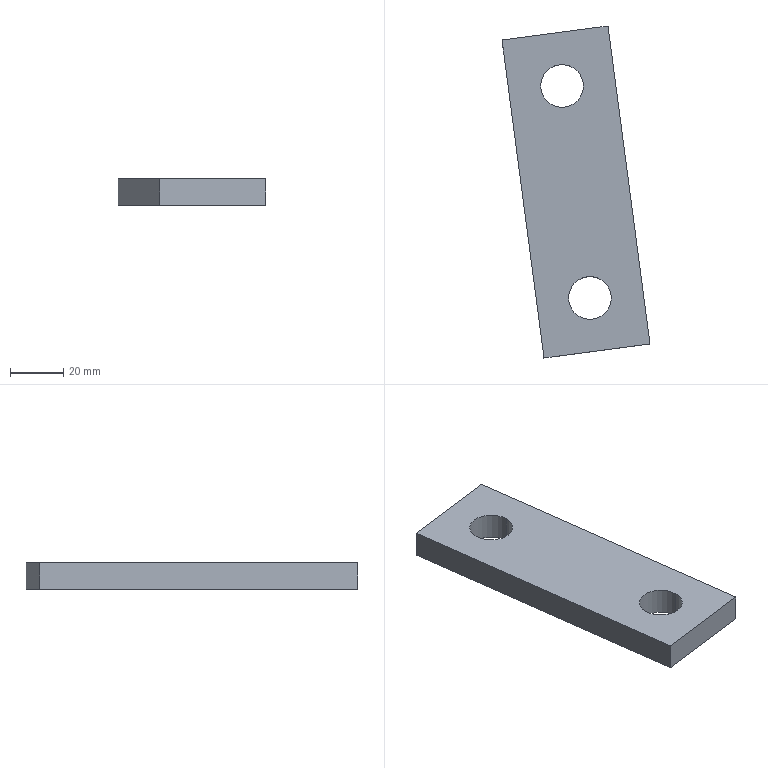Part | SolidWorks | features Extrusion 1 | 1 solid | 10 faces | box 55.334 x 124.197 x 10 mm | volume 43979 mm3 | plane 6 | cylinder 4 | commonest cylinder face diameters 16 x4
STEP:
#1=CARTESIAN_POINT('',(5154.359,2207.673,10.));
#2=VERTEX_POINT('',#1);
#3=CARTESIAN_POINT('',(5170.359,2207.673,10.));
#4=VERTEX_POINT('',#3);
#5=CARTESIAN_POINT('',(5162.359,2207.673,10.));
#6=DIRECTION('',(0.,0.,1.));
#7=DIRECTION('',(-1.,0.,0.));
#8=AXIS2_PLACEMENT_3D('',#5,#6,#7);
#9=CIRCLE('',#8,8.);
#10=EDGE_CURVE('',#2,#4,#9,.T.);
#11=ORIENTED_EDGE('',*,*,#10,.T.);
#12=CARTESIAN_POINT('',(5170.359,2207.673,0.));
#13=VERTEX_POINT('',#12);
#14=CARTESIAN_POINT('',(5170.359,2207.673,10.));
#15=DIRECTION('',(0.,0.,-1.));
#16=VECTOR('',#15,1000.);
#17=LINE('',#14,#16);
#18=EDGE_CURVE('',#4,#13,#17,.T.);
#19=ORIENTED_EDGE('',*,*,#18,.T.);
#20=CARTESIAN_POINT('',(5154.359,2207.673,0.));
#21=VERTEX_POINT('',#20);
#22=CARTESIAN_POINT('',(5162.359,2207.673,0.));
#23=DIRECTION('',(0.,0.,1.));
#24=DIRECTION('',(-1.,0.,0.));
#25=AXIS2_PLACEMENT_3D('',#22,#23,#24);
#26=CIRCLE('',#25,8.);
#27=EDGE_CURVE('',#21,#13,#26,.T.);
#28=ORIENTED_EDGE('',*,*,#27,.F.);
#29=CARTESIAN_POINT('',(5154.359,2207.673,10.));
#30=DIRECTION('',(0.,0.,-1.));
#31=VECTOR('',#30,1000.);
#32=LINE('',#29,#31);
#33=EDGE_CURVE('',#2,#21,#32,.T.);
#34=ORIENTED_EDGE('',*,*,#33,.F.);
#35=EDGE_LOOP('',(#11,#19,#28,#34));
#36=FACE_OUTER_BOUND('',#35,.T.);
#37=CARTESIAN_POINT('',(5162.359,2207.673,10.));
#38=DIRECTION('',(0.,0.,-1.));
#39=DIRECTION('',(-1.,0.,0.));
#40=AXIS2_PLACEMENT_3D('',#37,#38,#39);
#41=CYLINDRICAL_SURFACE('',#40,8.);
#42=ADVANCED_FACE('',(#36),#41,.F.);
#43=CARTESIAN_POINT('',(5143.908,2286.987,10.));
#44=VERTEX_POINT('',#43);
#45=CARTESIAN_POINT('',(5159.908,2286.987,10.));
#46=VERTEX_POINT('',#45);
#47=CARTESIAN_POINT('',(5151.908,2286.987,10.));
#48=DIRECTION('',(0.,0.,1.));
#49=DIRECTION('',(1.,0.,0.));
#50=AXIS2_PLACEMENT_3D('',#47,#48,#49);
#51=CIRCLE('',#50,8.);
#52=EDGE_CURVE('',#44,#46,#51,.T.);
#53=ORIENTED_EDGE('',*,*,#52,.T.);
#54=CARTESIAN_POINT('',(5159.908,2286.987,0.));
#55=VERTEX_POINT('',#54);
#56=CARTESIAN_POINT('',(5159.908,2286.987,10.));
#57=DIRECTION('',(0.,0.,-1.));
#58=VECTOR('',#57,1000.);
#59=LINE('',#56,#58);
#60=EDGE_CURVE('',#46,#55,#59,.T.);
#61=ORIENTED_EDGE('',*,*,#60,.T.);
#62=CARTESIAN_POINT('',(5143.908,2286.987,0.));
#63=VERTEX_POINT('',#62);
#64=CARTESIAN_POINT('',(5151.908,2286.987,0.));
#65=DIRECTION('',(0.,0.,1.));
#66=DIRECTION('',(1.,0.,0.));
#67=AXIS2_PLACEMENT_3D('',#64,#65,#66);
#68=CIRCLE('',#67,8.);
#69=EDGE_CURVE('',#63,#55,#68,.T.);
#70=ORIENTED_EDGE('',*,*,#69,.F.);
#71=CARTESIAN_POINT('',(5143.908,2286.987,10.));
#72=DIRECTION('',(0.,0.,-1.));
#73=VECTOR('',#72,1000.);
#74=LINE('',#71,#73);
#75=EDGE_CURVE('',#44,#63,#74,.T.);
#76=ORIENTED_EDGE('',*,*,#75,.F.);
#77=EDGE_LOOP('',(#53,#61,#70,#76));
#78=FACE_OUTER_BOUND('',#77,.T.);
#79=CARTESIAN_POINT('',(5151.908,2286.987,10.));
#80=DIRECTION('',(0.,0.,-1.));
#81=DIRECTION('',(-1.,0.,0.));
#82=AXIS2_PLACEMENT_3D('',#79,#80,#81);
#83=CYLINDRICAL_SURFACE('',#82,8.);
#84=ADVANCED_FACE('',(#78),#83,.F.);
#85=CARTESIAN_POINT('',(5129.467,2304.203,10.));
#86=VERTEX_POINT('',#85);
#87=CARTESIAN_POINT('',(5145.143,2185.231,10.));
#88=VERTEX_POINT('',#87);
#89=CARTESIAN_POINT('',(5145.143,2185.231,10.));
#90=DIRECTION('',(0.1306,-0.9914,0.));
#91=VECTOR('',#90,1000.);
#92=LINE('',#89,#91);
#93=EDGE_CURVE('',#86,#88,#92,.T.);
#94=ORIENTED_EDGE('',*,*,#93,.T.);
#95=CARTESIAN_POINT('',(5184.801,2190.457,10.));
#96=VERTEX_POINT('',#95);
#97=CARTESIAN_POINT('',(5184.801,2190.457,10.));
#98=DIRECTION('',(0.9914,0.1306,0.));
#99=VECTOR('',#98,1000.);
#100=LINE('',#97,#99);
#101=EDGE_CURVE('',#88,#96,#100,.T.);
#102=ORIENTED_EDGE('',*,*,#101,.T.);
#103=CARTESIAN_POINT('',(5169.124,2309.428,10.));
#104=VERTEX_POINT('',#103);
#105=CARTESIAN_POINT('',(5169.124,2309.428,10.));
#106=DIRECTION('',(-0.1306,0.9914,0.));
#107=VECTOR('',#106,1000.);
#108=LINE('',#105,#107);
#109=EDGE_CURVE('',#96,#104,#108,.T.);
#110=ORIENTED_EDGE('',*,*,#109,.T.);
#111=CARTESIAN_POINT('',(5129.467,2304.203,10.));
#112=DIRECTION('',(-0.9914,-0.1306,0.));
#113=VECTOR('',#112,1000.);
#114=LINE('',#111,#113);
#115=EDGE_CURVE('',#104,#86,#114,.T.);
#116=ORIENTED_EDGE('',*,*,#115,.T.);
#117=EDGE_LOOP('',(#94,#102,#110,#116));
#118=FACE_OUTER_BOUND('',#117,.T.);
#119=ORIENTED_EDGE('',*,*,#52,.F.);
#120=CARTESIAN_POINT('',(5151.908,2286.987,10.));
#121=DIRECTION('',(0.,0.,1.));
#122=DIRECTION('',(1.,0.,0.));
#123=AXIS2_PLACEMENT_3D('',#120,#121,#122);
#124=CIRCLE('',#123,8.);
#125=EDGE_CURVE('',#46,#44,#124,.T.);
#126=ORIENTED_EDGE('',*,*,#125,.F.);
#127=EDGE_LOOP('',(#119,#126));
#128=FACE_BOUND('',#127,.T.);
#129=ORIENTED_EDGE('',*,*,#10,.F.);
#130=CARTESIAN_POINT('',(5162.359,2207.673,10.));
#131=DIRECTION('',(0.,0.,1.));
#132=DIRECTION('',(-1.,0.,0.));
#133=AXIS2_PLACEMENT_3D('',#130,#131,#132);
#134=CIRCLE('',#133,8.);
#135=EDGE_CURVE('',#4,#2,#134,.T.);
#136=ORIENTED_EDGE('',*,*,#135,.F.);
#137=EDGE_LOOP('',(#129,#136));
#138=FACE_BOUND('',#137,.T.);
#139=CARTESIAN_POINT('',(0.,0.,10.));
#140=DIRECTION('',(0.,0.,-1.));
#141=DIRECTION('',(-1.,0.,0.));
#142=AXIS2_PLACEMENT_3D('',#139,#140,#141);
#143=PLANE('',#142);
#144=ADVANCED_FACE('',(#118,#128,#138),#143,.F.);
#145=ORIENTED_EDGE('',*,*,#69,.T.);
#146=CARTESIAN_POINT('',(5151.908,2286.987,0.));
#147=DIRECTION('',(0.,0.,1.));
#148=DIRECTION('',(1.,0.,0.));
#149=AXIS2_PLACEMENT_3D('',#146,#147,#148);
#150=CIRCLE('',#149,8.);
#151=EDGE_CURVE('',#55,#63,#150,.T.);
#152=ORIENTED_EDGE('',*,*,#151,.T.);
#153=EDGE_LOOP('',(#145,#152));
#154=FACE_BOUND('',#153,.T.);
#155=CARTESIAN_POINT('',(5145.143,2185.231,0.));
#156=VERTEX_POINT('',#155);
#157=CARTESIAN_POINT('',(5184.801,2190.457,0.));
#158=VERTEX_POINT('',#157);
#159=CARTESIAN_POINT('',(5184.801,2190.457,0.));
#160=DIRECTION('',(0.9914,0.1306,0.));
#161=VECTOR('',#160,1000.);
#162=LINE('',#159,#161);
#163=EDGE_CURVE('',#156,#158,#162,.T.);
#164=ORIENTED_EDGE('',*,*,#163,.F.);
#165=CARTESIAN_POINT('',(5129.467,2304.203,0.));
#166=VERTEX_POINT('',#165);
#167=CARTESIAN_POINT('',(5137.305,2244.717,0.));
#168=DIRECTION('',(0.1306,-0.9914,0.));
#169=VECTOR('',#168,1000.);
#170=LINE('',#167,#169);
#171=EDGE_CURVE('',#166,#156,#170,.T.);
#172=ORIENTED_EDGE('',*,*,#171,.F.);
#173=CARTESIAN_POINT('',(5169.124,2309.428,0.));
#174=VERTEX_POINT('',#173);
#175=CARTESIAN_POINT('',(5129.467,2304.203,0.));
#176=DIRECTION('',(-0.9914,-0.1306,0.));
#177=VECTOR('',#176,1000.);
#178=LINE('',#175,#177);
#179=EDGE_CURVE('',#174,#166,#178,.T.);
#180=ORIENTED_EDGE('',*,*,#179,.F.);
#181=CARTESIAN_POINT('',(5169.124,2309.428,0.));
#182=DIRECTION('',(-0.1306,0.9914,0.));
#183=VECTOR('',#182,1000.);
#184=LINE('',#181,#183);
#185=EDGE_CURVE('',#158,#174,#184,.T.);
#186=ORIENTED_EDGE('',*,*,#185,.F.);
#187=EDGE_LOOP('',(#164,#172,#180,#186));
#188=FACE_OUTER_BOUND('',#187,.T.);
#189=ORIENTED_EDGE('',*,*,#27,.T.);
#190=CARTESIAN_POINT('',(5162.359,2207.673,0.));
#191=DIRECTION('',(0.,0.,1.));
#192=DIRECTION('',(-1.,0.,0.));
#193=AXIS2_PLACEMENT_3D('',#190,#191,#192);
#194=CIRCLE('',#193,8.);
#195=EDGE_CURVE('',#13,#21,#194,.T.);
#196=ORIENTED_EDGE('',*,*,#195,.T.);
#197=EDGE_LOOP('',(#189,#196));
#198=FACE_BOUND('',#197,.T.);
#199=CARTESIAN_POINT('',(0.,0.,0.));
#200=DIRECTION('',(0.,0.,-1.));
#201=DIRECTION('',(-1.,0.,0.));
#202=AXIS2_PLACEMENT_3D('',#199,#200,#201);
#203=PLANE('',#202);
#204=ADVANCED_FACE('',(#154,#188,#198),#203,.T.);
#205=ORIENTED_EDGE('',*,*,#163,.T.);
#206=CARTESIAN_POINT('',(5184.801,2190.457,10.));
#207=DIRECTION('',(0.,0.,-1.));
#208=VECTOR('',#207,1000.);
#209=LINE('',#206,#208);
#210=EDGE_CURVE('',#96,#158,#209,.T.);
#211=ORIENTED_EDGE('',*,*,#210,.F.);
#212=ORIENTED_EDGE('',*,*,#101,.F.);
#213=CARTESIAN_POINT('',(5145.143,2185.231,10.));
#214=DIRECTION('',(0.,0.,-1.));
#215=VECTOR('',#214,1000.);
#216=LINE('',#213,#215);
#217=EDGE_CURVE('',#88,#156,#216,.T.);
#218=ORIENTED_EDGE('',*,*,#217,.T.);
#219=EDGE_LOOP('',(#205,#211,#212,#218));
#220=FACE_OUTER_BOUND('',#219,.T.);
#221=CARTESIAN_POINT('',(5184.801,2190.457,10.));
#222=DIRECTION('',(-0.1306,0.9914,0.));
#223=DIRECTION('',(-0.9914,-0.1306,0.));
#224=AXIS2_PLACEMENT_3D('',#221,#222,#223);
#225=PLANE('',#224);
#226=ADVANCED_FACE('',(#220),#225,.F.);
#227=ORIENTED_EDGE('',*,*,#185,.T.);
#228=CARTESIAN_POINT('',(5169.124,2309.428,10.));
#229=DIRECTION('',(0.,0.,-1.));
#230=VECTOR('',#229,1000.);
#231=LINE('',#228,#230);
#232=EDGE_CURVE('',#104,#174,#231,.T.);
#233=ORIENTED_EDGE('',*,*,#232,.F.);
#234=ORIENTED_EDGE('',*,*,#109,.F.);
#235=ORIENTED_EDGE('',*,*,#210,.T.);
#236=EDGE_LOOP('',(#227,#233,#234,#235));
#237=FACE_OUTER_BOUND('',#236,.T.);
#238=CARTESIAN_POINT('',(5169.124,2309.428,10.));
#239=DIRECTION('',(-0.9914,-0.1306,0.));
#240=DIRECTION('',(0.1306,-0.9914,0.));
#241=AXIS2_PLACEMENT_3D('',#238,#239,#240);
#242=PLANE('',#241);
#243=ADVANCED_FACE('',(#237),#242,.F.);
#244=ORIENTED_EDGE('',*,*,#179,.T.);
#245=CARTESIAN_POINT('',(5129.467,2304.203,10.));
#246=DIRECTION('',(0.,0.,-1.));
#247=VECTOR('',#246,1000.);
#248=LINE('',#245,#247);
#249=EDGE_CURVE('',#86,#166,#248,.T.);
#250=ORIENTED_EDGE('',*,*,#249,.F.);
#251=ORIENTED_EDGE('',*,*,#115,.F.);
#252=ORIENTED_EDGE('',*,*,#232,.T.);
#253=EDGE_LOOP('',(#244,#250,#251,#252));
#254=FACE_OUTER_BOUND('',#253,.T.);
#255=CARTESIAN_POINT('',(5129.467,2304.203,10.));
#256=DIRECTION('',(0.1306,-0.9914,0.));
#257=DIRECTION('',(0.9914,0.1306,0.));
#258=AXIS2_PLACEMENT_3D('',#255,#256,#257);
#259=PLANE('',#258);
#260=ADVANCED_FACE('',(#254),#259,.F.);
#261=ORIENTED_EDGE('',*,*,#171,.T.);
#262=ORIENTED_EDGE('',*,*,#217,.F.);
#263=ORIENTED_EDGE('',*,*,#93,.F.);
#264=ORIENTED_EDGE('',*,*,#249,.T.);
#265=EDGE_LOOP('',(#261,#262,#263,#264));
#266=FACE_OUTER_BOUND('',#265,.T.);
#267=CARTESIAN_POINT('',(5137.305,2244.717,10.));
#268=DIRECTION('',(0.9914,0.1306,0.));
#269=DIRECTION('',(-0.1306,0.9914,0.));
#270=AXIS2_PLACEMENT_3D('',#267,#268,#269);
#271=PLANE('',#270);
#272=ADVANCED_FACE('',(#266),#271,.F.);
#273=ORIENTED_EDGE('',*,*,#60,.F.);
#274=ORIENTED_EDGE('',*,*,#125,.T.);
#275=ORIENTED_EDGE('',*,*,#75,.T.);
#276=ORIENTED_EDGE('',*,*,#151,.F.);
#277=EDGE_LOOP('',(#273,#274,#275,#276));
#278=FACE_OUTER_BOUND('',#277,.T.);
#279=CARTESIAN_POINT('',(5151.908,2286.987,10.));
#280=DIRECTION('',(0.,0.,-1.));
#281=DIRECTION('',(-1.,0.,0.));
#282=AXIS2_PLACEMENT_3D('',#279,#280,#281);
#283=CYLINDRICAL_SURFACE('',#282,8.);
#284=ADVANCED_FACE('',(#278),#283,.F.);
#285=ORIENTED_EDGE('',*,*,#18,.F.);
#286=ORIENTED_EDGE('',*,*,#135,.T.);
#287=ORIENTED_EDGE('',*,*,#33,.T.);
#288=ORIENTED_EDGE('',*,*,#195,.F.);
#289=EDGE_LOOP('',(#285,#286,#287,#288));
#290=FACE_OUTER_BOUND('',#289,.T.);
#291=CARTESIAN_POINT('',(5162.359,2207.673,10.));
#292=DIRECTION('',(0.,0.,-1.));
#293=DIRECTION('',(-1.,0.,0.));
#294=AXIS2_PLACEMENT_3D('',#291,#292,#293);
#295=CYLINDRICAL_SURFACE('',#294,8.);
#296=ADVANCED_FACE('',(#290),#295,.F.);
#297=CLOSED_SHELL('',(#42,#84,#144,#204,#226,#243,#260,#272,#284,#296));
#298=MANIFOLD_SOLID_BREP('',#297);
#299=CARTESIAN_POINT('',(0.,0.,0.));
#300=DIRECTION('',(0.,0.,1.));
#301=DIRECTION('',(1.,0.,0.));
#302=AXIS2_PLACEMENT_3D('',#299,#300,#301);
#303=(LENGTH_UNIT()NAMED_UNIT(*)SI_UNIT(.MILLI.,.METRE.));
#304=UNCERTAINTY_MEASURE_WITH_UNIT(LENGTH_MEASURE(0.00001),#303,'','');
#305=(NAMED_UNIT(*)PLANE_ANGLE_UNIT()SI_UNIT($,.RADIAN.));
#306=(NAMED_UNIT(*)SI_UNIT($,.STERADIAN.)SOLID_ANGLE_UNIT());
#307=(GEOMETRIC_REPRESENTATION_CONTEXT(3)GLOBAL_UNCERTAINTY_ASSIGNED_CONTEXT((#304))GLOBAL_UNIT_ASSIGNED_CONTEXT((#303,#305,#306))REPRESENTATION_CONTEXT('',''));
#308=ADVANCED_BREP_SHAPE_REPRESENTATION('',(#298,#302),#307);